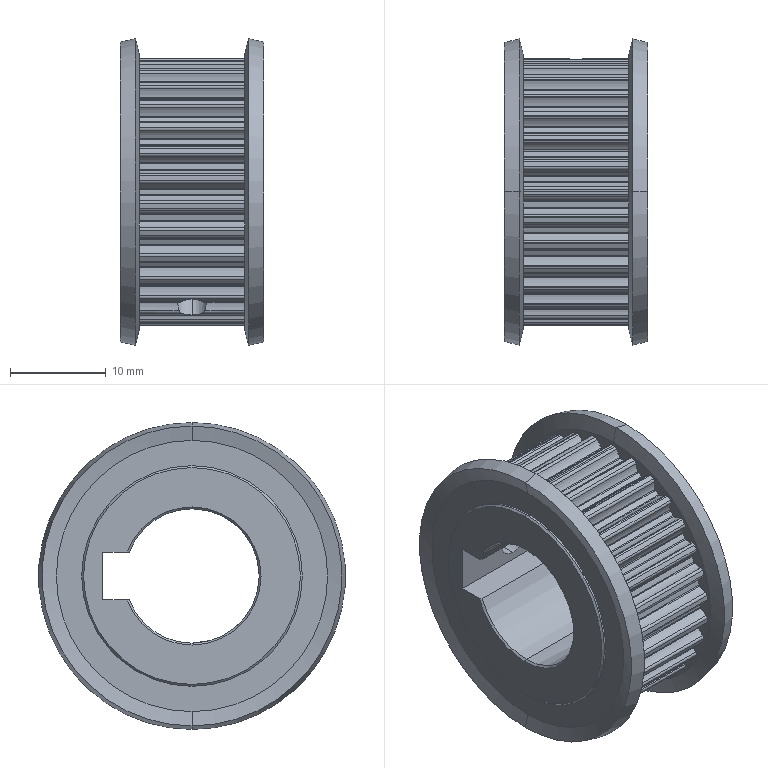Part | SolidWorks | features BaseBody 1 | 1 solid | 317 faces | box 15 x 32 x 32 mm | volume 6455 mm3 | cylinder 291 | cone 17 | plane 9 | commonest cylinder face diameters 0.56 x76 0.3 x73 3.95 x68 25.67 x32 27.89 x31 3.242 x4